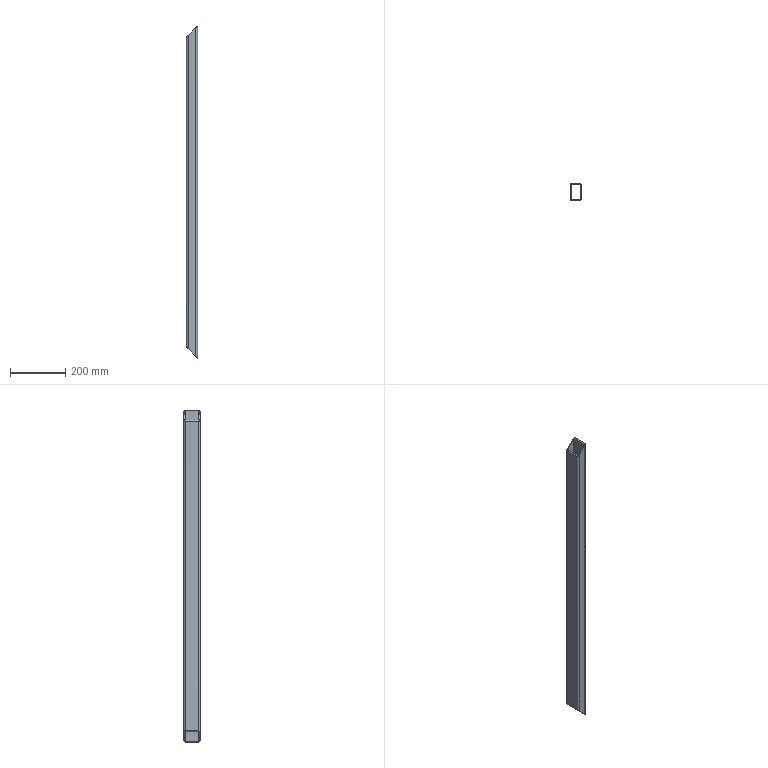Part | STEP file | Profile 40601200-1 | 1 solid | 18 faces | box 40 x 60 x 1200 mm | volume 664297 mm3 | plane 10 | cylinder 8 | commonest cylinder face diameters 6.4 x4 12.8 x4
STEP:
#1=CARTESIAN_POINT('',(40.,6.4,600.));
#2=VERTEX_POINT('',#1);
#3=CARTESIAN_POINT('',(40.,53.6,600.));
#4=VERTEX_POINT('',#3);
#5=CARTESIAN_POINT('',(40.,53.6,600.));
#6=DIRECTION('',(0.,1.,0.));
#7=VECTOR('',#6,1000.);
#8=LINE('',#5,#7);
#9=EDGE_CURVE('',#2,#4,#8,.T.);
#10=ORIENTED_EDGE('',*,*,#9,.F.);
#11=CARTESIAN_POINT('',(40.,6.4,-600.));
#12=VERTEX_POINT('',#11);
#13=CARTESIAN_POINT('',(40.,6.4,600.));
#14=DIRECTION('',(0.,0.,1.));
#15=VECTOR('',#14,1000.);
#16=LINE('',#13,#15);
#17=EDGE_CURVE('',#12,#2,#16,.T.);
#18=ORIENTED_EDGE('',*,*,#17,.F.);
#19=CARTESIAN_POINT('',(40.,53.6,-600.));
#20=VERTEX_POINT('',#19);
#21=CARTESIAN_POINT('',(40.,53.6,-600.));
#22=DIRECTION('',(0.,-1.,0.));
#23=VECTOR('',#22,1000.);
#24=LINE('',#21,#23);
#25=EDGE_CURVE('',#20,#12,#24,.T.);
#26=ORIENTED_EDGE('',*,*,#25,.F.);
#27=CARTESIAN_POINT('',(40.,53.6,600.));
#28=DIRECTION('',(0.,0.,-1.));
#29=VECTOR('',#28,1000.);
#30=LINE('',#27,#29);
#31=EDGE_CURVE('',#4,#20,#30,.T.);
#32=ORIENTED_EDGE('',*,*,#31,.F.);
#33=EDGE_LOOP('',(#10,#18,#26,#32));
#34=FACE_OUTER_BOUND('',#33,.T.);
#35=CARTESIAN_POINT('',(40.,53.6,600.));
#36=DIRECTION('',(-1.,0.,0.));
#37=DIRECTION('',(0.,0.,1.));
#38=AXIS2_PLACEMENT_3D('',#35,#36,#37);
#39=PLANE('',#38);
#40=ADVANCED_FACE('',(#34),#39,.F.);
#41=CARTESIAN_POINT('',(33.6,60.,-593.6));
#42=VERTEX_POINT('',#41);
#43=CARTESIAN_POINT('',(40.,53.6,-600.));
#44=CARTESIAN_POINT('',(40.,57.349,-600.));
#45=CARTESIAN_POINT('',(37.349,60.,-597.349));
#46=CARTESIAN_POINT('',(33.6,60.,-593.6));
#47=(BOUNDED_CURVE()B_SPLINE_CURVE(3,(#43,#44,#45,#46),.UNSPECIFIED.,.F.,.F.)B_SPLINE_CURVE_WITH_KNOTS((4,4),(0.,1.571),.UNSPECIFIED.)CURVE()GEOMETRIC_REPRESENTATION_ITEM()RATIONAL_B_SPLINE_CURVE((1.,0.8047,0.8047,1.))REPRESENTATION_ITEM(''));
#48=EDGE_CURVE('',#20,#42,#47,.T.);
#49=ORIENTED_EDGE('',*,*,#48,.T.);
#50=CARTESIAN_POINT('',(33.6,60.,593.6));
#51=VERTEX_POINT('',#50);
#52=CARTESIAN_POINT('',(33.6,60.,600.));
#53=DIRECTION('',(0.,0.,1.));
#54=VECTOR('',#53,1000.);
#55=LINE('',#52,#54);
#56=EDGE_CURVE('',#42,#51,#55,.T.);
#57=ORIENTED_EDGE('',*,*,#56,.T.);
#58=CARTESIAN_POINT('',(33.6,60.,593.6));
#59=CARTESIAN_POINT('',(37.349,60.,597.349));
#60=CARTESIAN_POINT('',(40.,57.349,600.));
#61=CARTESIAN_POINT('',(40.,53.6,600.));
#62=(BOUNDED_CURVE()B_SPLINE_CURVE(3,(#58,#59,#60,#61),.UNSPECIFIED.,.F.,.F.)B_SPLINE_CURVE_WITH_KNOTS((4,4),(1.571,3.142),.UNSPECIFIED.)CURVE()GEOMETRIC_REPRESENTATION_ITEM()RATIONAL_B_SPLINE_CURVE((1.,0.8047,0.8047,1.))REPRESENTATION_ITEM(''));
#63=EDGE_CURVE('',#51,#4,#62,.T.);
#64=ORIENTED_EDGE('',*,*,#63,.T.);
#65=ORIENTED_EDGE('',*,*,#31,.T.);
#66=EDGE_LOOP('',(#49,#57,#64,#65));
#67=FACE_OUTER_BOUND('',#66,.T.);
#68=CARTESIAN_POINT('',(33.6,53.6,600.));
#69=DIRECTION('',(0.,0.,-1.));
#70=DIRECTION('',(-1.,0.,0.));
#71=AXIS2_PLACEMENT_3D('',#68,#69,#70);
#72=CYLINDRICAL_SURFACE('',#71,6.4);
#73=ADVANCED_FACE('',(#67),#72,.T.);
#74=CARTESIAN_POINT('',(36.8,53.6,596.8));
#75=VERTEX_POINT('',#74);
#76=CARTESIAN_POINT('',(33.6,56.8,593.6));
#77=VERTEX_POINT('',#76);
#78=CARTESIAN_POINT('',(36.8,53.6,596.8));
#79=CARTESIAN_POINT('',(36.8,55.475,596.8));
#80=CARTESIAN_POINT('',(35.475,56.8,595.475));
#81=CARTESIAN_POINT('',(33.6,56.8,593.6));
#82=(BOUNDED_CURVE()B_SPLINE_CURVE(3,(#78,#79,#80,#81),.UNSPECIFIED.,.F.,.F.)B_SPLINE_CURVE_WITH_KNOTS((4,4),(3.142,4.712),.UNSPECIFIED.)CURVE()GEOMETRIC_REPRESENTATION_ITEM()RATIONAL_B_SPLINE_CURVE((1.,0.8047,0.8047,1.))REPRESENTATION_ITEM(''));
#83=EDGE_CURVE('',#75,#77,#82,.T.);
#84=ORIENTED_EDGE('',*,*,#83,.F.);
#85=CARTESIAN_POINT('',(36.8,6.4,596.8));
#86=VERTEX_POINT('',#85);
#87=CARTESIAN_POINT('',(36.8,0.,596.8));
#88=DIRECTION('',(0.,1.,0.));
#89=VECTOR('',#88,1000.);
#90=LINE('',#87,#89);
#91=EDGE_CURVE('',#86,#75,#90,.T.);
#92=ORIENTED_EDGE('',*,*,#91,.F.);
#93=CARTESIAN_POINT('',(33.6,3.2,593.6));
#94=VERTEX_POINT('',#93);
#95=CARTESIAN_POINT('',(33.6,3.2,593.6));
#96=CARTESIAN_POINT('',(35.475,3.2,595.475));
#97=CARTESIAN_POINT('',(36.8,4.525,596.8));
#98=CARTESIAN_POINT('',(36.8,6.4,596.8));
#99=(BOUNDED_CURVE()B_SPLINE_CURVE(3,(#95,#96,#97,#98),.UNSPECIFIED.,.F.,.F.)B_SPLINE_CURVE_WITH_KNOTS((4,4),(1.571,3.142),.UNSPECIFIED.)CURVE()GEOMETRIC_REPRESENTATION_ITEM()RATIONAL_B_SPLINE_CURVE((1.,0.8047,0.8047,1.))REPRESENTATION_ITEM(''));
#100=EDGE_CURVE('',#94,#86,#99,.T.);
#101=ORIENTED_EDGE('',*,*,#100,.F.);
#102=CARTESIAN_POINT('',(6.4,3.2,566.4));
#103=VERTEX_POINT('',#102);
#104=CARTESIAN_POINT('',(0.,3.2,560.));
#105=DIRECTION('',(0.7071,0.,0.7071));
#106=VECTOR('',#105,1000.);
#107=LINE('',#104,#106);
#108=EDGE_CURVE('',#103,#94,#107,.T.);
#109=ORIENTED_EDGE('',*,*,#108,.F.);
#110=CARTESIAN_POINT('',(3.2,6.4,563.2));
#111=VERTEX_POINT('',#110);
#112=CARTESIAN_POINT('',(3.2,6.4,563.2));
#113=CARTESIAN_POINT('',(3.2,4.525,563.2));
#114=CARTESIAN_POINT('',(4.525,3.2,564.525));
#115=CARTESIAN_POINT('',(6.4,3.2,566.4));
#116=(BOUNDED_CURVE()B_SPLINE_CURVE(3,(#112,#113,#114,#115),.UNSPECIFIED.,.F.,.F.)B_SPLINE_CURVE_WITH_KNOTS((4,4),(0.,1.571),.UNSPECIFIED.)CURVE()GEOMETRIC_REPRESENTATION_ITEM()RATIONAL_B_SPLINE_CURVE((1.,0.8047,0.8047,1.))REPRESENTATION_ITEM(''));
#117=EDGE_CURVE('',#111,#103,#116,.T.);
#118=ORIENTED_EDGE('',*,*,#117,.F.);
#119=CARTESIAN_POINT('',(3.2,53.6,563.2));
#120=VERTEX_POINT('',#119);
#121=CARTESIAN_POINT('',(3.2,0.,563.2));
#122=DIRECTION('',(0.,-1.,0.));
#123=VECTOR('',#122,1000.);
#124=LINE('',#121,#123);
#125=EDGE_CURVE('',#120,#111,#124,.T.);
#126=ORIENTED_EDGE('',*,*,#125,.F.);
#127=CARTESIAN_POINT('',(6.4,56.8,566.4));
#128=VERTEX_POINT('',#127);
#129=CARTESIAN_POINT('',(6.4,56.8,566.4));
#130=CARTESIAN_POINT('',(4.525,56.8,564.525));
#131=CARTESIAN_POINT('',(3.2,55.475,563.2));
#132=CARTESIAN_POINT('',(3.2,53.6,563.2));
#133=(BOUNDED_CURVE()B_SPLINE_CURVE(3,(#129,#130,#131,#132),.UNSPECIFIED.,.F.,.F.)B_SPLINE_CURVE_WITH_KNOTS((4,4),(4.712,6.283),.UNSPECIFIED.)CURVE()GEOMETRIC_REPRESENTATION_ITEM()RATIONAL_B_SPLINE_CURVE((1.,0.8047,0.8047,1.))REPRESENTATION_ITEM(''));
#134=EDGE_CURVE('',#128,#120,#133,.T.);
#135=ORIENTED_EDGE('',*,*,#134,.F.);
#136=CARTESIAN_POINT('',(0.,56.8,560.));
#137=DIRECTION('',(-0.7071,0.,-0.7071));
#138=VECTOR('',#137,1000.);
#139=LINE('',#136,#138);
#140=EDGE_CURVE('',#77,#128,#139,.T.);
#141=ORIENTED_EDGE('',*,*,#140,.F.);
#142=EDGE_LOOP('',(#84,#92,#101,#109,#118,#126,#135,#141));
#143=FACE_BOUND('',#142,.T.);
#144=ORIENTED_EDGE('',*,*,#9,.T.);
#145=ORIENTED_EDGE('',*,*,#63,.F.);
#146=CARTESIAN_POINT('',(6.4,60.,566.4));
#147=VERTEX_POINT('',#146);
#148=CARTESIAN_POINT('',(0.,60.,560.));
#149=DIRECTION('',(0.7071,0.,0.7071));
#150=VECTOR('',#149,1000.);
#151=LINE('',#148,#150);
#152=EDGE_CURVE('',#147,#51,#151,.T.);
#153=ORIENTED_EDGE('',*,*,#152,.F.);
#154=CARTESIAN_POINT('',(0.,53.6,560.));
#155=VERTEX_POINT('',#154);
#156=CARTESIAN_POINT('',(0.,53.6,560.));
#157=CARTESIAN_POINT('',(0.,57.349,560.));
#158=CARTESIAN_POINT('',(2.651,60.,562.651));
#159=CARTESIAN_POINT('',(6.4,60.,566.4));
#160=(BOUNDED_CURVE()B_SPLINE_CURVE(3,(#156,#157,#158,#159),.UNSPECIFIED.,.F.,.F.)B_SPLINE_CURVE_WITH_KNOTS((4,4),(0.,1.571),.UNSPECIFIED.)CURVE()GEOMETRIC_REPRESENTATION_ITEM()RATIONAL_B_SPLINE_CURVE((1.,0.8047,0.8047,1.))REPRESENTATION_ITEM(''));
#161=EDGE_CURVE('',#155,#147,#160,.T.);
#162=ORIENTED_EDGE('',*,*,#161,.F.);
#163=CARTESIAN_POINT('',(0.,6.4,560.));
#164=VERTEX_POINT('',#163);
#165=CARTESIAN_POINT('',(0.,0.,560.));
#166=DIRECTION('',(0.,1.,0.));
#167=VECTOR('',#166,1000.);
#168=LINE('',#165,#167);
#169=EDGE_CURVE('',#164,#155,#168,.T.);
#170=ORIENTED_EDGE('',*,*,#169,.F.);
#171=CARTESIAN_POINT('',(6.4,0.,566.4));
#172=VERTEX_POINT('',#171);
#173=CARTESIAN_POINT('',(6.4,0.,566.4));
#174=CARTESIAN_POINT('',(2.651,0.,562.651));
#175=CARTESIAN_POINT('',(0.,2.651,560.));
#176=CARTESIAN_POINT('',(0.,6.4,560.));
#177=(BOUNDED_CURVE()B_SPLINE_CURVE(3,(#173,#174,#175,#176),.UNSPECIFIED.,.F.,.F.)B_SPLINE_CURVE_WITH_KNOTS((4,4),(4.712,6.283),.UNSPECIFIED.)CURVE()GEOMETRIC_REPRESENTATION_ITEM()RATIONAL_B_SPLINE_CURVE((1.,0.8047,0.8047,1.))REPRESENTATION_ITEM(''));
#178=EDGE_CURVE('',#172,#164,#177,.T.);
#179=ORIENTED_EDGE('',*,*,#178,.F.);
#180=CARTESIAN_POINT('',(33.6,0.,593.6));
#181=VERTEX_POINT('',#180);
#182=CARTESIAN_POINT('',(0.,0.,560.));
#183=DIRECTION('',(-0.7071,0.,-0.7071));
#184=VECTOR('',#183,1000.);
#185=LINE('',#182,#184);
#186=EDGE_CURVE('',#181,#172,#185,.T.);
#187=ORIENTED_EDGE('',*,*,#186,.F.);
#188=CARTESIAN_POINT('',(40.,6.4,600.));
#189=CARTESIAN_POINT('',(40.,2.651,600.));
#190=CARTESIAN_POINT('',(37.349,0.,597.349));
#191=CARTESIAN_POINT('',(33.6,0.,593.6));
#192=(BOUNDED_CURVE()B_SPLINE_CURVE(3,(#188,#189,#190,#191),.UNSPECIFIED.,.F.,.F.)B_SPLINE_CURVE_WITH_KNOTS((4,4),(3.142,4.712),.UNSPECIFIED.)CURVE()GEOMETRIC_REPRESENTATION_ITEM()RATIONAL_B_SPLINE_CURVE((1.,0.8047,0.8047,1.))REPRESENTATION_ITEM(''));
#193=EDGE_CURVE('',#2,#181,#192,.T.);
#194=ORIENTED_EDGE('',*,*,#193,.F.);
#195=EDGE_LOOP('',(#144,#145,#153,#162,#170,#179,#187,#194));
#196=FACE_OUTER_BOUND('',#195,.T.);
#197=CARTESIAN_POINT('',(0.,0.,560.));
#198=DIRECTION('',(0.7071,0.,-0.7071));
#199=DIRECTION('',(-0.7071,0.,-0.7071));
#200=AXIS2_PLACEMENT_3D('',#197,#198,#199);
#201=PLANE('',#200);
#202=ADVANCED_FACE('',(#143,#196),#201,.F.);
#203=CARTESIAN_POINT('',(33.6,0.,-593.6));
#204=VERTEX_POINT('',#203);
#205=CARTESIAN_POINT('',(33.6,0.,-593.6));
#206=CARTESIAN_POINT('',(37.349,0.,-597.349));
#207=CARTESIAN_POINT('',(40.,2.651,-600.));
#208=CARTESIAN_POINT('',(40.,6.4,-600.));
#209=(BOUNDED_CURVE()B_SPLINE_CURVE(3,(#205,#206,#207,#208),.UNSPECIFIED.,.F.,.F.)B_SPLINE_CURVE_WITH_KNOTS((4,4),(4.712,6.283),.UNSPECIFIED.)CURVE()GEOMETRIC_REPRESENTATION_ITEM()RATIONAL_B_SPLINE_CURVE((1.,0.8047,0.8047,1.))REPRESENTATION_ITEM(''));
#210=EDGE_CURVE('',#204,#12,#209,.T.);
#211=ORIENTED_EDGE('',*,*,#210,.T.);
#212=ORIENTED_EDGE('',*,*,#17,.T.);
#213=ORIENTED_EDGE('',*,*,#193,.T.);
#214=CARTESIAN_POINT('',(33.6,0.,600.));
#215=DIRECTION('',(0.,0.,-1.));
#216=VECTOR('',#215,1000.);
#217=LINE('',#214,#216);
#218=EDGE_CURVE('',#181,#204,#217,.T.);
#219=ORIENTED_EDGE('',*,*,#218,.T.);
#220=EDGE_LOOP('',(#211,#212,#213,#219));
#221=FACE_OUTER_BOUND('',#220,.T.);
#222=CARTESIAN_POINT('',(33.6,6.4,600.));
#223=DIRECTION('',(0.,0.,-1.));
#224=DIRECTION('',(-1.,0.,0.));
#225=AXIS2_PLACEMENT_3D('',#222,#223,#224);
#226=CYLINDRICAL_SURFACE('',#225,6.4);
#227=ADVANCED_FACE('',(#221),#226,.T.);
#228=CARTESIAN_POINT('',(3.2,53.6,-563.2));
#229=VERTEX_POINT('',#228);
#230=CARTESIAN_POINT('',(6.4,56.8,-566.4));
#231=VERTEX_POINT('',#230);
#232=CARTESIAN_POINT('',(3.2,53.6,-563.2));
#233=CARTESIAN_POINT('',(3.2,55.475,-563.2));
#234=CARTESIAN_POINT('',(4.525,56.8,-564.525));
#235=CARTESIAN_POINT('',(6.4,56.8,-566.4));
#236=(BOUNDED_CURVE()B_SPLINE_CURVE(3,(#232,#233,#234,#235),.UNSPECIFIED.,.F.,.F.)B_SPLINE_CURVE_WITH_KNOTS((4,4),(3.142,4.712),.UNSPECIFIED.)CURVE()GEOMETRIC_REPRESENTATION_ITEM()RATIONAL_B_SPLINE_CURVE((1.,0.8047,0.8047,1.))REPRESENTATION_ITEM(''));
#237=EDGE_CURVE('',#229,#231,#236,.T.);
#238=ORIENTED_EDGE('',*,*,#237,.F.);
#239=CARTESIAN_POINT('',(3.2,6.4,-563.2));
#240=VERTEX_POINT('',#239);
#241=CARTESIAN_POINT('',(3.2,0.,-563.2));
#242=DIRECTION('',(0.,1.,0.));
#243=VECTOR('',#242,1000.);
#244=LINE('',#241,#243);
#245=EDGE_CURVE('',#240,#229,#244,.T.);
#246=ORIENTED_EDGE('',*,*,#245,.F.);
#247=CARTESIAN_POINT('',(6.4,3.2,-566.4));
#248=VERTEX_POINT('',#247);
#249=CARTESIAN_POINT('',(6.4,3.2,-566.4));
#250=CARTESIAN_POINT('',(4.525,3.2,-564.525));
#251=CARTESIAN_POINT('',(3.2,4.525,-563.2));
#252=CARTESIAN_POINT('',(3.2,6.4,-563.2));
#253=(BOUNDED_CURVE()B_SPLINE_CURVE(3,(#249,#250,#251,#252),.UNSPECIFIED.,.F.,.F.)B_SPLINE_CURVE_WITH_KNOTS((4,4),(1.571,3.142),.UNSPECIFIED.)CURVE()GEOMETRIC_REPRESENTATION_ITEM()RATIONAL_B_SPLINE_CURVE((1.,0.8047,0.8047,1.))REPRESENTATION_ITEM(''));
#254=EDGE_CURVE('',#248,#240,#253,.T.);
#255=ORIENTED_EDGE('',*,*,#254,.F.);
#256=CARTESIAN_POINT('',(33.6,3.2,-593.6));
#257=VERTEX_POINT('',#256);
#258=CARTESIAN_POINT('',(40.,3.2,-600.));
#259=DIRECTION('',(-0.7071,0.,0.7071));
#260=VECTOR('',#259,1000.);
#261=LINE('',#258,#260);
#262=EDGE_CURVE('',#257,#248,#261,.T.);
#263=ORIENTED_EDGE('',*,*,#262,.F.);
#264=CARTESIAN_POINT('',(36.8,6.4,-596.8));
#265=VERTEX_POINT('',#264);
#266=CARTESIAN_POINT('',(36.8,6.4,-596.8));
#267=CARTESIAN_POINT('',(36.8,4.525,-596.8));
#268=CARTESIAN_POINT('',(35.475,3.2,-595.475));
#269=CARTESIAN_POINT('',(33.6,3.2,-593.6));
#270=(BOUNDED_CURVE()B_SPLINE_CURVE(3,(#266,#267,#268,#269),.UNSPECIFIED.,.F.,.F.)B_SPLINE_CURVE_WITH_KNOTS((4,4),(0.,1.571),.UNSPECIFIED.)CURVE()GEOMETRIC_REPRESENTATION_ITEM()RATIONAL_B_SPLINE_CURVE((1.,0.8047,0.8047,1.))REPRESENTATION_ITEM(''));
#271=EDGE_CURVE('',#265,#257,#270,.T.);
#272=ORIENTED_EDGE('',*,*,#271,.F.);
#273=CARTESIAN_POINT('',(36.8,53.6,-596.8));
#274=VERTEX_POINT('',#273);
#275=CARTESIAN_POINT('',(36.8,0.,-596.8));
#276=DIRECTION('',(0.,-1.,0.));
#277=VECTOR('',#276,1000.);
#278=LINE('',#275,#277);
#279=EDGE_CURVE('',#274,#265,#278,.T.);
#280=ORIENTED_EDGE('',*,*,#279,.F.);
#281=CARTESIAN_POINT('',(33.6,56.8,-593.6));
#282=VERTEX_POINT('',#281);
#283=CARTESIAN_POINT('',(33.6,56.8,-593.6));
#284=CARTESIAN_POINT('',(35.475,56.8,-595.475));
#285=CARTESIAN_POINT('',(36.8,55.475,-596.8));
#286=CARTESIAN_POINT('',(36.8,53.6,-596.8));
#287=(BOUNDED_CURVE()B_SPLINE_CURVE(3,(#283,#284,#285,#286),.UNSPECIFIED.,.F.,.F.)B_SPLINE_CURVE_WITH_KNOTS((4,4),(4.712,6.283),.UNSPECIFIED.)CURVE()GEOMETRIC_REPRESENTATION_ITEM()RATIONAL_B_SPLINE_CURVE((1.,0.8047,0.8047,1.))REPRESENTATION_ITEM(''));
#288=EDGE_CURVE('',#282,#274,#287,.T.);
#289=ORIENTED_EDGE('',*,*,#288,.F.);
#290=CARTESIAN_POINT('',(40.,56.8,-600.));
#291=DIRECTION('',(0.7071,0.,-0.7071));
#292=VECTOR('',#291,1000.);
#293=LINE('',#290,#292);
#294=EDGE_CURVE('',#231,#282,#293,.T.);
#295=ORIENTED_EDGE('',*,*,#294,.F.);
#296=EDGE_LOOP('',(#238,#246,#255,#263,#272,#280,#289,#295));
#297=FACE_BOUND('',#296,.T.);
#298=CARTESIAN_POINT('',(6.4,0.,-566.4));
#299=VERTEX_POINT('',#298);
#300=CARTESIAN_POINT('',(40.,0.,-600.));
#301=DIRECTION('',(0.7071,0.,-0.7071));
#302=VECTOR('',#301,1000.);
#303=LINE('',#300,#302);
#304=EDGE_CURVE('',#299,#204,#303,.T.);
#305=ORIENTED_EDGE('',*,*,#304,.F.);
#306=CARTESIAN_POINT('',(0.,6.4,-560.));
#307=VERTEX_POINT('',#306);
#308=CARTESIAN_POINT('',(0.,6.4,-560.));
#309=CARTESIAN_POINT('',(0.,2.651,-560.));
#310=CARTESIAN_POINT('',(2.651,0.,-562.651));
#311=CARTESIAN_POINT('',(6.4,0.,-566.4));
#312=(BOUNDED_CURVE()B_SPLINE_CURVE(3,(#308,#309,#310,#311),.UNSPECIFIED.,.F.,.T.)B_SPLINE_CURVE_WITH_KNOTS((4,4),(3.142,4.712),.UNSPECIFIED.)CURVE()GEOMETRIC_REPRESENTATION_ITEM()RATIONAL_B_SPLINE_CURVE((1.,0.8047,0.8047,1.))REPRESENTATION_ITEM(''));
#313=EDGE_CURVE('',#307,#299,#312,.T.);
#314=ORIENTED_EDGE('',*,*,#313,.F.);
#315=CARTESIAN_POINT('',(0.,53.6,-560.));
#316=VERTEX_POINT('',#315);
#317=CARTESIAN_POINT('',(0.,0.,-560.));
#318=DIRECTION('',(0.,-1.,0.));
#319=VECTOR('',#318,1000.);
#320=LINE('',#317,#319);
#321=EDGE_CURVE('',#316,#307,#320,.T.);
#322=ORIENTED_EDGE('',*,*,#321,.F.);
#323=CARTESIAN_POINT('',(6.4,60.,-566.4));
#324=VERTEX_POINT('',#323);
#325=CARTESIAN_POINT('',(6.4,60.,-566.4));
#326=CARTESIAN_POINT('',(2.651,60.,-562.651));
#327=CARTESIAN_POINT('',(0.,57.349,-560.));
#328=CARTESIAN_POINT('',(0.,53.6,-560.));
#329=(BOUNDED_CURVE()B_SPLINE_CURVE(3,(#325,#326,#327,#328),.UNSPECIFIED.,.F.,.F.)B_SPLINE_CURVE_WITH_KNOTS((4,4),(1.571,3.142),.UNSPECIFIED.)CURVE()GEOMETRIC_REPRESENTATION_ITEM()RATIONAL_B_SPLINE_CURVE((1.,0.8047,0.8047,1.))REPRESENTATION_ITEM(''));
#330=EDGE_CURVE('',#324,#316,#329,.T.);
#331=ORIENTED_EDGE('',*,*,#330,.F.);
#332=CARTESIAN_POINT('',(40.,60.,-600.));
#333=DIRECTION('',(-0.7071,0.,0.7071));
#334=VECTOR('',#333,1000.);
#335=LINE('',#332,#334);
#336=EDGE_CURVE('',#42,#324,#335,.T.);
#337=ORIENTED_EDGE('',*,*,#336,.F.);
#338=ORIENTED_EDGE('',*,*,#48,.F.);
#339=ORIENTED_EDGE('',*,*,#25,.T.);
#340=ORIENTED_EDGE('',*,*,#210,.F.);
#341=EDGE_LOOP('',(#305,#314,#322,#331,#337,#338,#339,#340));
#342=FACE_OUTER_BOUND('',#341,.T.);
#343=CARTESIAN_POINT('',(40.,0.,-600.));
#344=DIRECTION('',(0.7071,0.,0.7071));
#345=DIRECTION('',(0.7071,0.,-0.7071));
#346=AXIS2_PLACEMENT_3D('',#343,#344,#345);
#347=PLANE('',#346);
#348=ADVANCED_FACE('',(#297,#342),#347,.F.);
#349=ORIENTED_EDGE('',*,*,#152,.T.);
#350=ORIENTED_EDGE('',*,*,#56,.F.);
#351=ORIENTED_EDGE('',*,*,#336,.T.);
#352=CARTESIAN_POINT('',(6.4,60.,600.));
#353=DIRECTION('',(0.,0.,-1.));
#354=VECTOR('',#353,1000.);
#355=LINE('',#352,#354);
#356=EDGE_CURVE('',#147,#324,#355,.T.);
#357=ORIENTED_EDGE('',*,*,#356,.F.);
#358=EDGE_LOOP('',(#349,#350,#351,#357));
#359=FACE_OUTER_BOUND('',#358,.T.);
#360=CARTESIAN_POINT('',(33.6,60.,600.));
#361=DIRECTION('',(0.,-1.,0.));
#362=DIRECTION('',(0.,0.,-1.));
#363=AXIS2_PLACEMENT_3D('',#360,#361,#362);
#364=PLANE('',#363);
#365=ADVANCED_FACE('',(#359),#364,.F.);
#366=ORIENTED_EDGE('',*,*,#294,.T.);
#367=CARTESIAN_POINT('',(33.6,56.8,600.));
#368=DIRECTION('',(0.,0.,1.));
#369=VECTOR('',#368,1000.);
#370=LINE('',#367,#369);
#371=EDGE_CURVE('',#282,#77,#370,.T.);
#372=ORIENTED_EDGE('',*,*,#371,.T.);
#373=ORIENTED_EDGE('',*,*,#140,.T.);
#374=CARTESIAN_POINT('',(6.4,56.8,600.));
#375=DIRECTION('',(0.,0.,-1.));
#376=VECTOR('',#375,1000.);
#377=LINE('',#374,#376);
#378=EDGE_CURVE('',#128,#231,#377,.T.);
#379=ORIENTED_EDGE('',*,*,#378,.T.);
#380=EDGE_LOOP('',(#366,#372,#373,#379));
#381=FACE_OUTER_BOUND('',#380,.T.);
#382=CARTESIAN_POINT('',(33.6,56.8,600.));
#383=DIRECTION('',(0.,-1.,0.));
#384=DIRECTION('',(0.,0.,-1.));
#385=AXIS2_PLACEMENT_3D('',#382,#383,#384);
#386=PLANE('',#385);
#387=ADVANCED_FACE('',(#381),#386,.T.);
#388=ORIENTED_EDGE('',*,*,#83,.T.);
#389=ORIENTED_EDGE('',*,*,#371,.F.);
#390=ORIENTED_EDGE('',*,*,#288,.T.);
#391=CARTESIAN_POINT('',(36.8,53.6,600.));
#392=DIRECTION('',(0.,0.,-1.));
#393=VECTOR('',#392,1000.);
#394=LINE('',#391,#393);
#395=EDGE_CURVE('',#75,#274,#394,.T.);
#396=ORIENTED_EDGE('',*,*,#395,.F.);
#397=EDGE_LOOP('',(#388,#389,#390,#396));
#398=FACE_OUTER_BOUND('',#397,.T.);
#399=CARTESIAN_POINT('',(33.6,53.6,600.));
#400=DIRECTION('',(0.,0.,-1.));
#401=DIRECTION('',(-1.,0.,0.));
#402=AXIS2_PLACEMENT_3D('',#399,#400,#401);
#403=CYLINDRICAL_SURFACE('',#402,3.2);
#404=ADVANCED_FACE('',(#398),#403,.F.);
#405=ORIENTED_EDGE('',*,*,#279,.T.);
#406=CARTESIAN_POINT('',(36.8,6.4,600.));
#407=DIRECTION('',(0.,0.,1.));
#408=VECTOR('',#407,1000.);
#409=LINE('',#406,#408);
#410=EDGE_CURVE('',#265,#86,#409,.T.);
#411=ORIENTED_EDGE('',*,*,#410,.T.);
#412=ORIENTED_EDGE('',*,*,#91,.T.);
#413=ORIENTED_EDGE('',*,*,#395,.T.);
#414=EDGE_LOOP('',(#405,#411,#412,#413));
#415=FACE_OUTER_BOUND('',#414,.T.);
#416=CARTESIAN_POINT('',(36.8,53.6,600.));
#417=DIRECTION('',(-1.,0.,0.));
#418=DIRECTION('',(0.,0.,1.));
#419=AXIS2_PLACEMENT_3D('',#416,#417,#418);
#420=PLANE('',#419);
#421=ADVANCED_FACE('',(#415),#420,.T.);
#422=ORIENTED_EDGE('',*,*,#100,.T.);
#423=ORIENTED_EDGE('',*,*,#410,.F.);
#424=ORIENTED_EDGE('',*,*,#271,.T.);
#425=CARTESIAN_POINT('',(33.6,3.2,600.));
#426=DIRECTION('',(0.,0.,-1.));
#427=VECTOR('',#426,1000.);
#428=LINE('',#425,#427);
#429=EDGE_CURVE('',#94,#257,#428,.T.);
#430=ORIENTED_EDGE('',*,*,#429,.F.);
#431=EDGE_LOOP('',(#422,#423,#424,#430));
#432=FACE_OUTER_BOUND('',#431,.T.);
#433=CARTESIAN_POINT('',(33.6,6.4,600.));
#434=DIRECTION('',(0.,0.,-1.));
#435=DIRECTION('',(-1.,0.,0.));
#436=AXIS2_PLACEMENT_3D('',#433,#434,#435);
#437=CYLINDRICAL_SURFACE('',#436,3.2);
#438=ADVANCED_FACE('',(#432),#437,.F.);
#439=ORIENTED_EDGE('',*,*,#262,.T.);
#440=CARTESIAN_POINT('',(6.4,3.2,600.));
#441=DIRECTION('',(0.,0.,1.));
#442=VECTOR('',#441,1000.);
#443=LINE('',#440,#442);
#444=EDGE_CURVE('',#248,#103,#443,.T.);
#445=ORIENTED_EDGE('',*,*,#444,.T.);
#446=ORIENTED_EDGE('',*,*,#108,.T.);
#447=ORIENTED_EDGE('',*,*,#429,.T.);
#448=EDGE_LOOP('',(#439,#445,#446,#447));
#449=FACE_OUTER_BOUND('',#448,.T.);
#450=CARTESIAN_POINT('',(6.4,3.2,600.));
#451=DIRECTION('',(0.,1.,0.));
#452=DIRECTION('',(-1.,0.,0.));
#453=AXIS2_PLACEMENT_3D('',#450,#451,#452);
#454=PLANE('',#453);
#455=ADVANCED_FACE('',(#449),#454,.T.);
#456=ORIENTED_EDGE('',*,*,#117,.T.);
#457=ORIENTED_EDGE('',*,*,#444,.F.);
#458=ORIENTED_EDGE('',*,*,#254,.T.);
#459=CARTESIAN_POINT('',(3.2,6.4,600.));
#460=DIRECTION('',(0.,0.,-1.));
#461=VECTOR('',#460,1000.);
#462=LINE('',#459,#461);
#463=EDGE_CURVE('',#111,#240,#462,.T.);
#464=ORIENTED_EDGE('',*,*,#463,.F.);
#465=EDGE_LOOP('',(#456,#457,#458,#464));
#466=FACE_OUTER_BOUND('',#465,.T.);
#467=CARTESIAN_POINT('',(6.4,6.4,600.));
#468=DIRECTION('',(0.,0.,-1.));
#469=DIRECTION('',(-1.,0.,0.));
#470=AXIS2_PLACEMENT_3D('',#467,#468,#469);
#471=CYLINDRICAL_SURFACE('',#470,3.2);
#472=ADVANCED_FACE('',(#466),#471,.F.);
#473=ORIENTED_EDGE('',*,*,#245,.T.);
#474=CARTESIAN_POINT('',(3.2,53.6,600.));
#475=DIRECTION('',(0.,0.,1.));
#476=VECTOR('',#475,1000.);
#477=LINE('',#474,#476);
#478=EDGE_CURVE('',#229,#120,#477,.T.);
#479=ORIENTED_EDGE('',*,*,#478,.T.);
#480=ORIENTED_EDGE('',*,*,#125,.T.);
#481=ORIENTED_EDGE('',*,*,#463,.T.);
#482=EDGE_LOOP('',(#473,#479,#480,#481));
#483=FACE_OUTER_BOUND('',#482,.T.);
#484=CARTESIAN_POINT('',(3.2,6.4,600.));
#485=DIRECTION('',(1.,0.,0.));
#486=DIRECTION('',(0.,1.,0.));
#487=AXIS2_PLACEMENT_3D('',#484,#485,#486);
#488=PLANE('',#487);
#489=ADVANCED_FACE('',(#483),#488,.T.);
#490=ORIENTED_EDGE('',*,*,#134,.T.);
#491=ORIENTED_EDGE('',*,*,#478,.F.);
#492=ORIENTED_EDGE('',*,*,#237,.T.);
#493=ORIENTED_EDGE('',*,*,#378,.F.);
#494=EDGE_LOOP('',(#490,#491,#492,#493));
#495=FACE_OUTER_BOUND('',#494,.T.);
#496=CARTESIAN_POINT('',(6.4,53.6,600.));
#497=DIRECTION('',(0.,0.,-1.));
#498=DIRECTION('',(-1.,0.,0.));
#499=AXIS2_PLACEMENT_3D('',#496,#497,#498);
#500=CYLINDRICAL_SURFACE('',#499,3.2);
#501=ADVANCED_FACE('',(#495),#500,.F.);
#502=ORIENTED_EDGE('',*,*,#330,.T.);
#503=CARTESIAN_POINT('',(0.,53.6,600.));
#504=DIRECTION('',(0.,0.,1.));
#505=VECTOR('',#504,1000.);
#506=LINE('',#503,#505);
#507=EDGE_CURVE('',#316,#155,#506,.T.);
#508=ORIENTED_EDGE('',*,*,#507,.T.);
#509=ORIENTED_EDGE('',*,*,#161,.T.);
#510=ORIENTED_EDGE('',*,*,#356,.T.);
#511=EDGE_LOOP('',(#502,#508,#509,#510));
#512=FACE_OUTER_BOUND('',#511,.T.);
#513=CARTESIAN_POINT('',(6.4,53.6,600.));
#514=DIRECTION('',(0.,0.,-1.));
#515=DIRECTION('',(-1.,0.,0.));
#516=AXIS2_PLACEMENT_3D('',#513,#514,#515);
#517=CYLINDRICAL_SURFACE('',#516,6.4);
#518=ADVANCED_FACE('',(#512),#517,.T.);
#519=ORIENTED_EDGE('',*,*,#169,.T.);
#520=ORIENTED_EDGE('',*,*,#507,.F.);
#521=ORIENTED_EDGE('',*,*,#321,.T.);
#522=CARTESIAN_POINT('',(0.,6.4,600.));
#523=DIRECTION('',(0.,0.,-1.));
#524=VECTOR('',#523,1000.);
#525=LINE('',#522,#524);
#526=EDGE_CURVE('',#164,#307,#525,.T.);
#527=ORIENTED_EDGE('',*,*,#526,.F.);
#528=EDGE_LOOP('',(#519,#520,#521,#527));
#529=FACE_OUTER_BOUND('',#528,.T.);
#530=CARTESIAN_POINT('',(0.,6.4,600.));
#531=DIRECTION('',(1.,0.,0.));
#532=DIRECTION('',(0.,1.,0.));
#533=AXIS2_PLACEMENT_3D('',#530,#531,#532);
#534=PLANE('',#533);
#535=ADVANCED_FACE('',(#529),#534,.F.);
#536=ORIENTED_EDGE('',*,*,#313,.T.);
#537=CARTESIAN_POINT('',(6.4,0.,600.));
#538=DIRECTION('',(0.,0.,1.));
#539=VECTOR('',#538,1000.);
#540=LINE('',#537,#539);
#541=EDGE_CURVE('',#299,#172,#540,.T.);
#542=ORIENTED_EDGE('',*,*,#541,.T.);
#543=ORIENTED_EDGE('',*,*,#178,.T.);
#544=ORIENTED_EDGE('',*,*,#526,.T.);
#545=EDGE_LOOP('',(#536,#542,#543,#544));
#546=FACE_OUTER_BOUND('',#545,.T.);
#547=CARTESIAN_POINT('',(6.4,6.4,600.));
#548=DIRECTION('',(0.,0.,-1.));
#549=DIRECTION('',(-1.,0.,0.));
#550=AXIS2_PLACEMENT_3D('',#547,#548,#549);
#551=CYLINDRICAL_SURFACE('',#550,6.4);
#552=ADVANCED_FACE('',(#546),#551,.T.);
#553=ORIENTED_EDGE('',*,*,#186,.T.);
#554=ORIENTED_EDGE('',*,*,#541,.F.);
#555=ORIENTED_EDGE('',*,*,#304,.T.);
#556=ORIENTED_EDGE('',*,*,#218,.F.);
#557=EDGE_LOOP('',(#553,#554,#555,#556));
#558=FACE_OUTER_BOUND('',#557,.T.);
#559=CARTESIAN_POINT('',(6.4,0.,600.));
#560=DIRECTION('',(0.,1.,0.));
#561=DIRECTION('',(-1.,0.,0.));
#562=AXIS2_PLACEMENT_3D('',#559,#560,#561);
#563=PLANE('',#562);
#564=ADVANCED_FACE('',(#558),#563,.F.);
#565=CLOSED_SHELL('',(#40,#73,#202,#227,#348,#365,#387,#404,#421,#438,#455,#472,#489,#501,#518,#535,#552,#564));
#566=MANIFOLD_SOLID_BREP('',#565);
#567=CARTESIAN_POINT('',(0.,0.,0.));
#568=DIRECTION('',(0.,0.,1.));
#569=DIRECTION('',(1.,0.,0.));
#570=AXIS2_PLACEMENT_3D('',#567,#568,#569);
#571=(LENGTH_UNIT()NAMED_UNIT(*)SI_UNIT(.MILLI.,.METRE.));
#572=UNCERTAINTY_MEASURE_WITH_UNIT(LENGTH_MEASURE(0.00001),#571,'','');
#573=(NAMED_UNIT(*)PLANE_ANGLE_UNIT()SI_UNIT($,.RADIAN.));
#574=(NAMED_UNIT(*)SI_UNIT($,.STERADIAN.)SOLID_ANGLE_UNIT());
#575=(GEOMETRIC_REPRESENTATION_CONTEXT(3)GLOBAL_UNCERTAINTY_ASSIGNED_CONTEXT((#572))GLOBAL_UNIT_ASSIGNED_CONTEXT((#571,#573,#574))REPRESENTATION_CONTEXT('',''));
#576=ADVANCED_BREP_SHAPE_REPRESENTATION('',(#566,#570),#575);